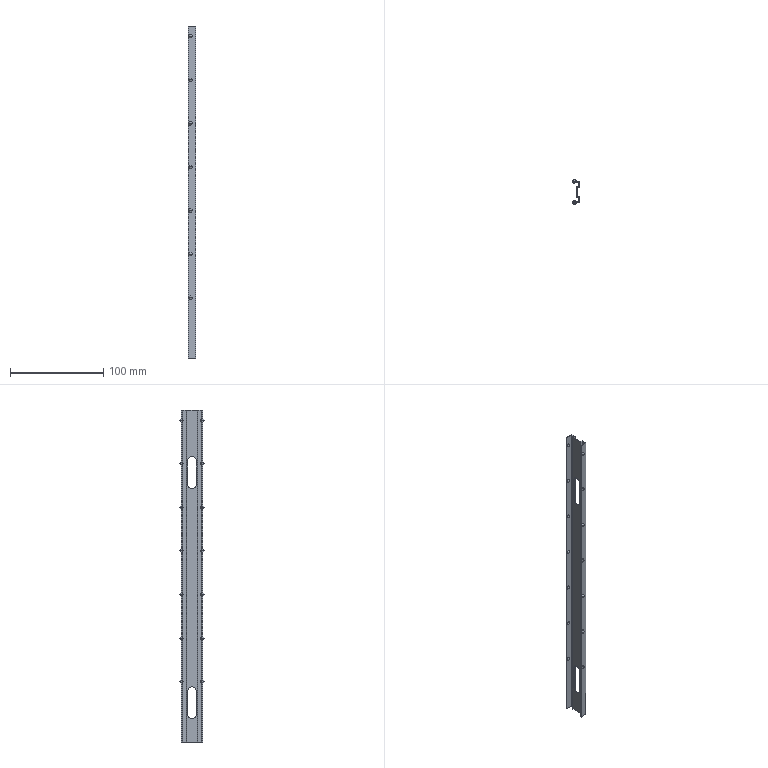Part | SolidWorks | features BaseBody 1, RefAxis 1 | 1 solid | 77 faces | box 7.8 x 26 x 355.6 mm | volume 9914 mm3 | spline 49 | plane 22 | cylinder 6 | commonest cylinder face diameters 9 x6